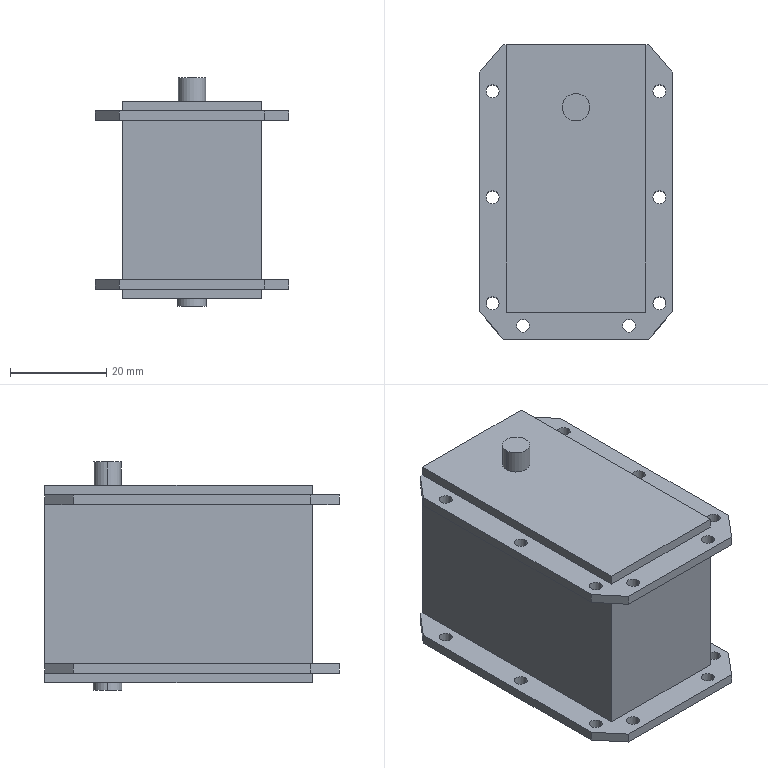Part | SolidWorks | features BaseBody 1 | 1 solid | 77 faces | box 40.2 x 61.1 x 47.35 mm | volume 68973 mm3 | cylinder 42 | plane 35 | commonest cylinder face diameters 2.7 x32 3.2 x2 5.7 x2 6 x2 8 x2 13 x2